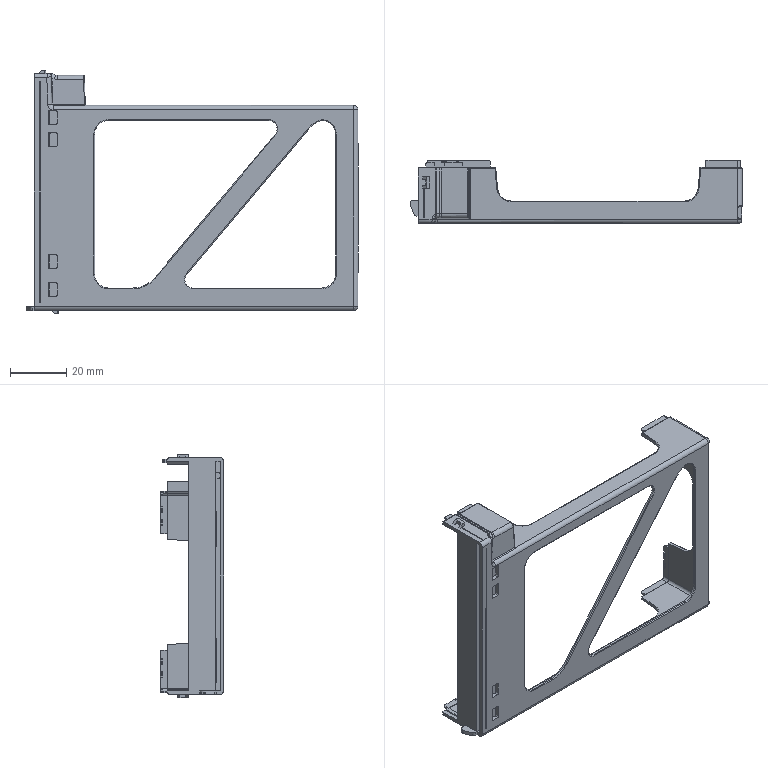Part | SolidWorks | features BaseBody 1 | 1 solid | 417 faces | box 118.5 x 22.6 x 87 mm | volume 22903 mm3 | plane 244 | cylinder 129 | spline 41 | torus 3 | commonest cylinder face diameters 1 x48 0.6 x33 3 x14 2 x13 10 x10 0.4 x2